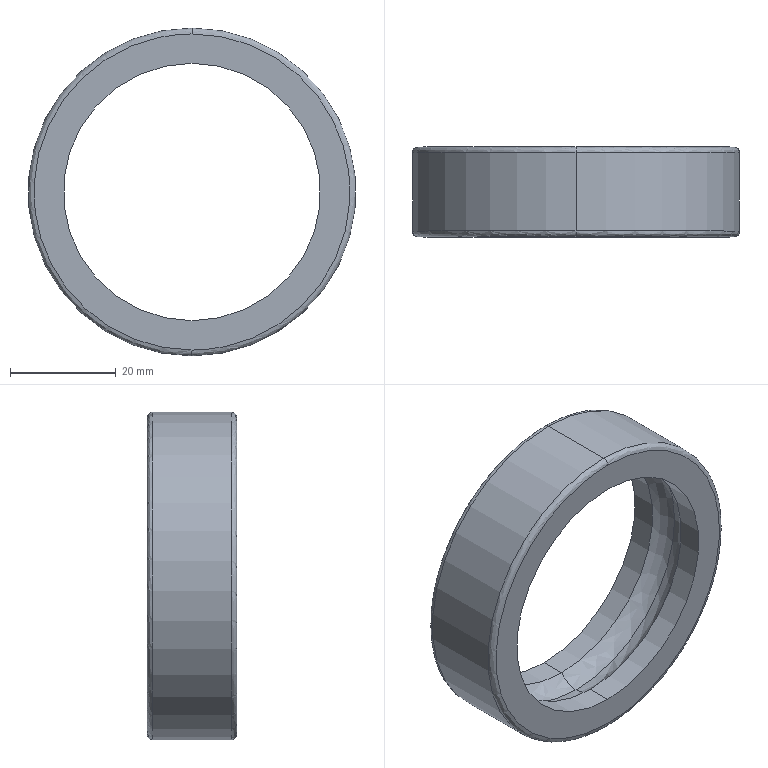Part | SolidWorks | features BaseBody 1 | 1 solid | 16 faces | box 62 x 17 x 62 mm | volume 17853 mm3 | spline 8 | cylinder 6 | plane 2 | commonest cylinder face diameters 48.68 x4 62 x2
STEP:
#1=CARTESIAN_POINT('',(0.,-8.5,29.9));
#2=VERTEX_POINT('',#1);
#3=CARTESIAN_POINT('',(0.,-8.5,-29.9));
#4=VERTEX_POINT('',#3);
#5=CARTESIAN_POINT('',(0.,-8.5,29.9));
#6=CARTESIAN_POINT('',(59.8,-8.5,29.9));
#7=CARTESIAN_POINT('',(59.8,-8.5,-29.9));
#8=CARTESIAN_POINT('',(0.,-8.5,-29.9));
#9=(BOUNDED_CURVE()B_SPLINE_CURVE(3,(#5,#6,#7,#8),.UNSPECIFIED.,.F.,.F.)B_SPLINE_CURVE_WITH_KNOTS((4,4),(0.,1.),.UNSPECIFIED.)CURVE()GEOMETRIC_REPRESENTATION_ITEM()RATIONAL_B_SPLINE_CURVE((1.,0.3333,0.3333,1.))REPRESENTATION_ITEM(''));
#10=EDGE_CURVE('',#2,#4,#9,.T.);
#11=ORIENTED_EDGE('',*,*,#10,.T.);
#12=CARTESIAN_POINT('',(0.,-7.4,-31.));
#13=VERTEX_POINT('',#12);
#14=CARTESIAN_POINT('',(0.,-7.4,-29.9));
#15=DIRECTION('',(1.,0.,0.));
#16=DIRECTION('',(0.,0.,-1.));
#17=AXIS2_PLACEMENT_3D('',#14,#15,#16);
#18=CIRCLE('',#17,1.1);
#19=EDGE_CURVE('',#4,#13,#18,.T.);
#20=ORIENTED_EDGE('',*,*,#19,.T.);
#21=CARTESIAN_POINT('',(0.,-7.4,31.));
#22=VERTEX_POINT('',#21);
#23=CARTESIAN_POINT('',(0.,-7.4,0.));
#24=DIRECTION('',(0.,1.,0.));
#25=DIRECTION('',(0.,0.,-1.));
#26=AXIS2_PLACEMENT_3D('',#23,#24,#25);
#27=CIRCLE('',#26,31.);
#28=EDGE_CURVE('',#22,#13,#27,.T.);
#29=ORIENTED_EDGE('',*,*,#28,.F.);
#30=CARTESIAN_POINT('',(0.,-7.4,29.9));
#31=DIRECTION('',(-1.,0.,0.));
#32=DIRECTION('',(0.,0.,1.));
#33=AXIS2_PLACEMENT_3D('',#30,#31,#32);
#34=CIRCLE('',#33,1.1);
#35=EDGE_CURVE('',#2,#22,#34,.T.);
#36=ORIENTED_EDGE('',*,*,#35,.F.);
#37=EDGE_LOOP('',(#11,#20,#29,#36));
#38=FACE_OUTER_BOUND('',#37,.T.);
#39=CARTESIAN_POINT('',(0.,-8.5,-29.9));
#40=CARTESIAN_POINT('',(59.8,-8.5,-29.9));
#41=CARTESIAN_POINT('',(59.8,-8.5,29.9));
#42=CARTESIAN_POINT('',(0.,-8.5,29.9));
#43=CARTESIAN_POINT('',(0.,-8.5,-30.544));
#44=CARTESIAN_POINT('',(61.089,-8.5,-30.544));
#45=CARTESIAN_POINT('',(61.089,-8.5,30.544));
#46=CARTESIAN_POINT('',(0.,-8.5,30.544));
#47=CARTESIAN_POINT('',(0.,-8.044,-31.));
#48=CARTESIAN_POINT('',(62.,-8.044,-31.));
#49=CARTESIAN_POINT('',(62.,-8.044,31.));
#50=CARTESIAN_POINT('',(0.,-8.044,31.));
#51=CARTESIAN_POINT('',(0.,-7.4,-31.));
#52=CARTESIAN_POINT('',(62.,-7.4,-31.));
#53=CARTESIAN_POINT('',(62.,-7.4,31.));
#54=CARTESIAN_POINT('',(0.,-7.4,31.));
#55=(BOUNDED_SURFACE()B_SPLINE_SURFACE(3,3,((#39,#40,#41,#42),(#43,#44,#45,#46),(#47,#48,#49,#50),(#51,#52,#53,#54)),.UNSPECIFIED.,.F.,.F.,.T.)B_SPLINE_SURFACE_WITH_KNOTS((4,4),(4,4),(0.,1.),(0.,1.),.UNSPECIFIED.)GEOMETRIC_REPRESENTATION_ITEM()RATIONAL_B_SPLINE_SURFACE(((1.,0.3333,0.3333,1.),(0.8047,0.2682,0.2682,0.8047),(0.8047,0.2682,0.2682,0.8047),(1.,0.3333,0.3333,1.)))REPRESENTATION_ITEM('')SURFACE());
#56=ADVANCED_FACE('',(#38),#55,.T.);
#57=CARTESIAN_POINT('',(0.,7.4,-31.));
#58=VERTEX_POINT('',#57);
#59=CARTESIAN_POINT('',(0.,7.4,31.));
#60=VERTEX_POINT('',#59);
#61=CARTESIAN_POINT('',(0.,7.4,0.));
#62=DIRECTION('',(0.,-1.,0.));
#63=DIRECTION('',(0.,0.,-1.));
#64=AXIS2_PLACEMENT_3D('',#61,#62,#63);
#65=CIRCLE('',#64,31.);
#66=EDGE_CURVE('',#58,#60,#65,.T.);
#67=ORIENTED_EDGE('',*,*,#66,.F.);
#68=CARTESIAN_POINT('',(0.,8.5,-29.9));
#69=VERTEX_POINT('',#68);
#70=CARTESIAN_POINT('',(0.,7.4,-29.9));
#71=DIRECTION('',(1.,0.,0.));
#72=DIRECTION('',(0.,0.,-1.));
#73=AXIS2_PLACEMENT_3D('',#70,#71,#72);
#74=CIRCLE('',#73,1.1);
#75=EDGE_CURVE('',#58,#69,#74,.T.);
#76=ORIENTED_EDGE('',*,*,#75,.T.);
#77=CARTESIAN_POINT('',(0.,8.5,29.9));
#78=VERTEX_POINT('',#77);
#79=CARTESIAN_POINT('',(0.,8.5,-29.9));
#80=CARTESIAN_POINT('',(59.8,8.5,-29.9));
#81=CARTESIAN_POINT('',(59.8,8.5,29.9));
#82=CARTESIAN_POINT('',(0.,8.5,29.9));
#83=(BOUNDED_CURVE()B_SPLINE_CURVE(3,(#79,#80,#81,#82),.UNSPECIFIED.,.F.,.F.)B_SPLINE_CURVE_WITH_KNOTS((4,4),(0.,1.),.UNSPECIFIED.)CURVE()GEOMETRIC_REPRESENTATION_ITEM()RATIONAL_B_SPLINE_CURVE((1.,0.3333,0.3333,1.))REPRESENTATION_ITEM(''));
#84=EDGE_CURVE('',#69,#78,#83,.T.);
#85=ORIENTED_EDGE('',*,*,#84,.T.);
#86=CARTESIAN_POINT('',(0.,7.4,29.9));
#87=DIRECTION('',(-1.,0.,0.));
#88=DIRECTION('',(0.,0.,1.));
#89=AXIS2_PLACEMENT_3D('',#86,#87,#88);
#90=CIRCLE('',#89,1.1);
#91=EDGE_CURVE('',#60,#78,#90,.T.);
#92=ORIENTED_EDGE('',*,*,#91,.F.);
#93=EDGE_LOOP('',(#67,#76,#85,#92));
#94=FACE_OUTER_BOUND('',#93,.T.);
#95=CARTESIAN_POINT('',(0.,7.4,-31.));
#96=CARTESIAN_POINT('',(62.,7.4,-31.));
#97=CARTESIAN_POINT('',(62.,7.4,31.));
#98=CARTESIAN_POINT('',(0.,7.4,31.));
#99=CARTESIAN_POINT('',(0.,8.044,-31.));
#100=CARTESIAN_POINT('',(62.,8.044,-31.));
#101=CARTESIAN_POINT('',(62.,8.044,31.));
#102=CARTESIAN_POINT('',(0.,8.044,31.));
#103=CARTESIAN_POINT('',(0.,8.5,-30.544));
#104=CARTESIAN_POINT('',(61.089,8.5,-30.544));
#105=CARTESIAN_POINT('',(61.089,8.5,30.544));
#106=CARTESIAN_POINT('',(0.,8.5,30.544));
#107=CARTESIAN_POINT('',(0.,8.5,-29.9));
#108=CARTESIAN_POINT('',(59.8,8.5,-29.9));
#109=CARTESIAN_POINT('',(59.8,8.5,29.9));
#110=CARTESIAN_POINT('',(0.,8.5,29.9));
#111=(BOUNDED_SURFACE()B_SPLINE_SURFACE(3,3,((#95,#96,#97,#98),(#99,#100,#101,#102),(#103,#104,#105,#106),(#107,#108,#109,#110)),.UNSPECIFIED.,.F.,.F.,.T.)B_SPLINE_SURFACE_WITH_KNOTS((4,4),(4,4),(0.,1.),(0.,1.),.UNSPECIFIED.)GEOMETRIC_REPRESENTATION_ITEM()RATIONAL_B_SPLINE_SURFACE(((1.,0.3333,0.3333,1.),(0.8047,0.2682,0.2682,0.8047),(0.8047,0.2682,0.2682,0.8047),(1.,0.3333,0.3333,1.)))REPRESENTATION_ITEM('')SURFACE());
#112=ADVANCED_FACE('',(#94),#111,.T.);
#113=CARTESIAN_POINT('',(0.,-3.832,24.34));
#114=VERTEX_POINT('',#113);
#115=CARTESIAN_POINT('',(0.,-3.832,-24.34));
#116=VERTEX_POINT('',#115);
#117=CARTESIAN_POINT('',(0.,-3.832,0.));
#118=DIRECTION('',(0.,-1.,0.));
#119=DIRECTION('',(0.,0.,-1.));
#120=AXIS2_PLACEMENT_3D('',#117,#118,#119);
#121=CIRCLE('',#120,24.34);
#122=EDGE_CURVE('',#114,#116,#121,.T.);
#123=ORIENTED_EDGE('',*,*,#122,.T.);
#124=CARTESIAN_POINT('',(0.,0.,-26.375));
#125=VERTEX_POINT('',#124);
#126=CARTESIAN_POINT('',(0.,0.,-21.75));
#127=DIRECTION('',(1.,0.,0.));
#128=DIRECTION('',(0.,0.,-1.));
#129=AXIS2_PLACEMENT_3D('',#126,#127,#128);
#130=CIRCLE('',#129,4.625);
#131=EDGE_CURVE('',#116,#125,#130,.T.);
#132=ORIENTED_EDGE('',*,*,#131,.T.);
#133=CARTESIAN_POINT('',(0.,0.,26.375));
#134=VERTEX_POINT('',#133);
#135=CARTESIAN_POINT('',(0.,0.,0.));
#136=DIRECTION('',(0.,-1.,0.));
#137=DIRECTION('',(0.,0.,1.));
#138=AXIS2_PLACEMENT_3D('',#135,#136,#137);
#139=CIRCLE('',#138,26.375);
#140=EDGE_CURVE('',#134,#125,#139,.T.);
#141=ORIENTED_EDGE('',*,*,#140,.F.);
#142=CARTESIAN_POINT('',(0.,0.,21.75));
#143=DIRECTION('',(-1.,0.,0.));
#144=DIRECTION('',(0.,0.,1.));
#145=AXIS2_PLACEMENT_3D('',#142,#143,#144);
#146=CIRCLE('',#145,4.625);
#147=EDGE_CURVE('',#114,#134,#146,.T.);
#148=ORIENTED_EDGE('',*,*,#147,.F.);
#149=EDGE_LOOP('',(#123,#132,#141,#148));
#150=FACE_OUTER_BOUND('',#149,.T.);
#151=CARTESIAN_POINT('',(0.,-3.832,24.34));
#152=CARTESIAN_POINT('',(-48.68,-3.832,24.34));
#153=CARTESIAN_POINT('',(-48.68,-3.832,-24.34));
#154=CARTESIAN_POINT('',(0.,-3.832,-24.34));
#155=CARTESIAN_POINT('',(0.,-2.953,25.639));
#156=CARTESIAN_POINT('',(-51.279,-2.953,25.639));
#157=CARTESIAN_POINT('',(-51.279,-2.953,-25.639));
#158=CARTESIAN_POINT('',(0.,-2.953,-25.639));
#159=CARTESIAN_POINT('',(0.,-1.568,26.375));
#160=CARTESIAN_POINT('',(-52.75,-1.568,26.375));
#161=CARTESIAN_POINT('',(-52.75,-1.568,-26.375));
#162=CARTESIAN_POINT('',(0.,-1.568,-26.375));
#163=CARTESIAN_POINT('',(0.,0.,26.375));
#164=CARTESIAN_POINT('',(-52.75,0.,26.375));
#165=CARTESIAN_POINT('',(-52.75,0.,-26.375));
#166=CARTESIAN_POINT('',(0.,0.,-26.375));
#167=(BOUNDED_SURFACE()B_SPLINE_SURFACE(3,3,((#151,#152,#153,#154),(#155,#156,#157,#158),(#159,#160,#161,#162),(#163,#164,#165,#166)),.UNSPECIFIED.,.F.,.F.,.F.)B_SPLINE_SURFACE_WITH_KNOTS((4,4),(4,4),(0.,1.),(0.,1.),.UNSPECIFIED.)GEOMETRIC_REPRESENTATION_ITEM()RATIONAL_B_SPLINE_SURFACE(((1.,0.3333,0.3333,1.),(0.9221,0.3074,0.3074,0.9221),(0.9221,0.3074,0.3074,0.9221),(1.,0.3333,0.3333,1.)))REPRESENTATION_ITEM('')SURFACE());
#168=ADVANCED_FACE('',(#150),#167,.F.);
#169=ORIENTED_EDGE('',*,*,#140,.T.);
#170=CARTESIAN_POINT('',(0.,3.832,-24.34));
#171=VERTEX_POINT('',#170);
#172=CARTESIAN_POINT('',(0.,0.,-21.75));
#173=DIRECTION('',(1.,0.,0.));
#174=DIRECTION('',(0.,0.,-1.));
#175=AXIS2_PLACEMENT_3D('',#172,#173,#174);
#176=CIRCLE('',#175,4.625);
#177=EDGE_CURVE('',#125,#171,#176,.T.);
#178=ORIENTED_EDGE('',*,*,#177,.T.);
#179=CARTESIAN_POINT('',(0.,3.832,24.34));
#180=VERTEX_POINT('',#179);
#181=CARTESIAN_POINT('',(0.,3.832,0.));
#182=DIRECTION('',(0.,1.,0.));
#183=DIRECTION('',(0.,0.,-1.));
#184=AXIS2_PLACEMENT_3D('',#181,#182,#183);
#185=CIRCLE('',#184,24.34);
#186=EDGE_CURVE('',#171,#180,#185,.T.);
#187=ORIENTED_EDGE('',*,*,#186,.T.);
#188=CARTESIAN_POINT('',(0.,0.,21.75));
#189=DIRECTION('',(-1.,0.,0.));
#190=DIRECTION('',(0.,0.,1.));
#191=AXIS2_PLACEMENT_3D('',#188,#189,#190);
#192=CIRCLE('',#191,4.625);
#193=EDGE_CURVE('',#134,#180,#192,.T.);
#194=ORIENTED_EDGE('',*,*,#193,.F.);
#195=EDGE_LOOP('',(#169,#178,#187,#194));
#196=FACE_OUTER_BOUND('',#195,.T.);
#197=CARTESIAN_POINT('',(0.,0.,26.375));
#198=CARTESIAN_POINT('',(-52.75,0.,26.375));
#199=CARTESIAN_POINT('',(-52.75,0.,-26.375));
#200=CARTESIAN_POINT('',(0.,0.,-26.375));
#201=CARTESIAN_POINT('',(0.,1.568,26.375));
#202=CARTESIAN_POINT('',(-52.75,1.568,26.375));
#203=CARTESIAN_POINT('',(-52.75,1.568,-26.375));
#204=CARTESIAN_POINT('',(0.,1.568,-26.375));
#205=CARTESIAN_POINT('',(0.,2.953,25.639));
#206=CARTESIAN_POINT('',(-51.279,2.953,25.639));
#207=CARTESIAN_POINT('',(-51.279,2.953,-25.639));
#208=CARTESIAN_POINT('',(0.,2.953,-25.639));
#209=CARTESIAN_POINT('',(0.,3.832,24.34));
#210=CARTESIAN_POINT('',(-48.68,3.832,24.34));
#211=CARTESIAN_POINT('',(-48.68,3.832,-24.34));
#212=CARTESIAN_POINT('',(0.,3.832,-24.34));
#213=(BOUNDED_SURFACE()B_SPLINE_SURFACE(3,3,((#197,#198,#199,#200),(#201,#202,#203,#204),(#205,#206,#207,#208),(#209,#210,#211,#212)),.UNSPECIFIED.,.F.,.F.,.T.)B_SPLINE_SURFACE_WITH_KNOTS((4,4),(4,4),(0.,1.),(0.,1.),.UNSPECIFIED.)GEOMETRIC_REPRESENTATION_ITEM()RATIONAL_B_SPLINE_SURFACE(((1.,0.3333,0.3333,1.),(0.9221,0.3074,0.3074,0.9221),(0.9221,0.3074,0.3074,0.9221),(1.,0.3333,0.3333,1.)))REPRESENTATION_ITEM('')SURFACE());
#214=ADVANCED_FACE('',(#196),#213,.F.);
#215=ORIENTED_EDGE('',*,*,#66,.T.);
#216=CARTESIAN_POINT('',(0.,9.35,31.));
#217=DIRECTION('',(0.,-1.,0.));
#218=VECTOR('',#217,1000.);
#219=LINE('',#216,#218);
#220=EDGE_CURVE('',#60,#22,#219,.T.);
#221=ORIENTED_EDGE('',*,*,#220,.T.);
#222=ORIENTED_EDGE('',*,*,#28,.T.);
#223=CARTESIAN_POINT('',(0.,9.35,-31.));
#224=DIRECTION('',(0.,-1.,0.));
#225=VECTOR('',#224,1000.);
#226=LINE('',#223,#225);
#227=EDGE_CURVE('',#58,#13,#226,.T.);
#228=ORIENTED_EDGE('',*,*,#227,.F.);
#229=EDGE_LOOP('',(#215,#221,#222,#228));
#230=FACE_OUTER_BOUND('',#229,.T.);
#231=CARTESIAN_POINT('',(0.,9.35,0.));
#232=DIRECTION('',(0.,-1.,0.));
#233=DIRECTION('',(0.,0.,-1.));
#234=AXIS2_PLACEMENT_3D('',#231,#232,#233);
#235=CYLINDRICAL_SURFACE('',#234,31.);
#236=ADVANCED_FACE('',(#230),#235,.T.);
#237=ORIENTED_EDGE('',*,*,#122,.F.);
#238=CARTESIAN_POINT('',(0.,-8.5,24.34));
#239=VERTEX_POINT('',#238);
#240=CARTESIAN_POINT('',(0.,9.35,24.34));
#241=DIRECTION('',(0.,-1.,0.));
#242=VECTOR('',#241,1000.);
#243=LINE('',#240,#242);
#244=EDGE_CURVE('',#114,#239,#243,.T.);
#245=ORIENTED_EDGE('',*,*,#244,.T.);
#246=CARTESIAN_POINT('',(0.,-8.5,-24.34));
#247=VERTEX_POINT('',#246);
#248=CARTESIAN_POINT('',(0.,-8.5,0.));
#249=DIRECTION('',(0.,1.,0.));
#250=DIRECTION('',(0.,0.,-1.));
#251=AXIS2_PLACEMENT_3D('',#248,#249,#250);
#252=CIRCLE('',#251,24.34);
#253=EDGE_CURVE('',#247,#239,#252,.T.);
#254=ORIENTED_EDGE('',*,*,#253,.F.);
#255=CARTESIAN_POINT('',(0.,9.35,-24.34));
#256=DIRECTION('',(0.,-1.,0.));
#257=VECTOR('',#256,1000.);
#258=LINE('',#255,#257);
#259=EDGE_CURVE('',#116,#247,#258,.T.);
#260=ORIENTED_EDGE('',*,*,#259,.F.);
#261=EDGE_LOOP('',(#237,#245,#254,#260));
#262=FACE_OUTER_BOUND('',#261,.T.);
#263=CARTESIAN_POINT('',(0.,9.35,0.));
#264=DIRECTION('',(0.,-1.,0.));
#265=DIRECTION('',(0.,0.,-1.));
#266=AXIS2_PLACEMENT_3D('',#263,#264,#265);
#267=CYLINDRICAL_SURFACE('',#266,24.34);
#268=ADVANCED_FACE('',(#262),#267,.F.);
#269=CARTESIAN_POINT('',(0.,8.5,-24.34));
#270=VERTEX_POINT('',#269);
#271=CARTESIAN_POINT('',(0.,8.5,24.34));
#272=VERTEX_POINT('',#271);
#273=CARTESIAN_POINT('',(0.,8.5,0.));
#274=DIRECTION('',(0.,1.,0.));
#275=DIRECTION('',(0.,0.,-1.));
#276=AXIS2_PLACEMENT_3D('',#273,#274,#275);
#277=CIRCLE('',#276,24.34);
#278=EDGE_CURVE('',#270,#272,#277,.T.);
#279=ORIENTED_EDGE('',*,*,#278,.T.);
#280=CARTESIAN_POINT('',(0.,9.35,24.34));
#281=DIRECTION('',(0.,-1.,0.));
#282=VECTOR('',#281,1000.);
#283=LINE('',#280,#282);
#284=EDGE_CURVE('',#272,#180,#283,.T.);
#285=ORIENTED_EDGE('',*,*,#284,.T.);
#286=ORIENTED_EDGE('',*,*,#186,.F.);
#287=CARTESIAN_POINT('',(0.,9.35,-24.34));
#288=DIRECTION('',(0.,-1.,0.));
#289=VECTOR('',#288,1000.);
#290=LINE('',#287,#289);
#291=EDGE_CURVE('',#270,#171,#290,.T.);
#292=ORIENTED_EDGE('',*,*,#291,.F.);
#293=EDGE_LOOP('',(#279,#285,#286,#292));
#294=FACE_OUTER_BOUND('',#293,.T.);
#295=CARTESIAN_POINT('',(0.,9.35,0.));
#296=DIRECTION('',(0.,-1.,0.));
#297=DIRECTION('',(0.,0.,-1.));
#298=AXIS2_PLACEMENT_3D('',#295,#296,#297);
#299=CYLINDRICAL_SURFACE('',#298,24.34);
#300=ADVANCED_FACE('',(#294),#299,.F.);
#301=ORIENTED_EDGE('',*,*,#177,.F.);
#302=CARTESIAN_POINT('',(0.,0.,0.));
#303=DIRECTION('',(0.,-1.,0.));
#304=DIRECTION('',(0.,0.,1.));
#305=AXIS2_PLACEMENT_3D('',#302,#303,#304);
#306=CIRCLE('',#305,26.375);
#307=EDGE_CURVE('',#125,#134,#306,.T.);
#308=ORIENTED_EDGE('',*,*,#307,.T.);
#309=ORIENTED_EDGE('',*,*,#193,.T.);
#310=CARTESIAN_POINT('',(0.,3.832,0.));
#311=DIRECTION('',(0.,1.,0.));
#312=DIRECTION('',(0.,0.,-1.));
#313=AXIS2_PLACEMENT_3D('',#310,#311,#312);
#314=CIRCLE('',#313,24.34);
#315=EDGE_CURVE('',#180,#171,#314,.T.);
#316=ORIENTED_EDGE('',*,*,#315,.T.);
#317=EDGE_LOOP('',(#301,#308,#309,#316));
#318=FACE_OUTER_BOUND('',#317,.T.);
#319=CARTESIAN_POINT('',(0.,0.,-26.375));
#320=CARTESIAN_POINT('',(52.75,0.,-26.375));
#321=CARTESIAN_POINT('',(52.75,0.,26.375));
#322=CARTESIAN_POINT('',(0.,0.,26.375));
#323=CARTESIAN_POINT('',(0.,1.568,-26.375));
#324=CARTESIAN_POINT('',(52.75,1.568,-26.375));
#325=CARTESIAN_POINT('',(52.75,1.568,26.375));
#326=CARTESIAN_POINT('',(0.,1.568,26.375));
#327=CARTESIAN_POINT('',(0.,2.953,-25.639));
#328=CARTESIAN_POINT('',(51.279,2.953,-25.639));
#329=CARTESIAN_POINT('',(51.279,2.953,25.639));
#330=CARTESIAN_POINT('',(0.,2.953,25.639));
#331=CARTESIAN_POINT('',(0.,3.832,-24.34));
#332=CARTESIAN_POINT('',(48.68,3.832,-24.34));
#333=CARTESIAN_POINT('',(48.68,3.832,24.34));
#334=CARTESIAN_POINT('',(0.,3.832,24.34));
#335=(BOUNDED_SURFACE()B_SPLINE_SURFACE(3,3,((#319,#320,#321,#322),(#323,#324,#325,#326),(#327,#328,#329,#330),(#331,#332,#333,#334)),.UNSPECIFIED.,.F.,.F.,.T.)B_SPLINE_SURFACE_WITH_KNOTS((4,4),(4,4),(0.,1.),(0.,1.),.UNSPECIFIED.)GEOMETRIC_REPRESENTATION_ITEM()RATIONAL_B_SPLINE_SURFACE(((1.,0.3333,0.3333,1.),(0.9221,0.3074,0.3074,0.9221),(0.9221,0.3074,0.3074,0.9221),(1.,0.3333,0.3333,1.)))REPRESENTATION_ITEM('')SURFACE());
#336=ADVANCED_FACE('',(#318),#335,.F.);
#337=ORIENTED_EDGE('',*,*,#220,.F.);
#338=CARTESIAN_POINT('',(0.,7.4,0.));
#339=DIRECTION('',(0.,-1.,0.));
#340=DIRECTION('',(0.,0.,-1.));
#341=AXIS2_PLACEMENT_3D('',#338,#339,#340);
#342=CIRCLE('',#341,31.);
#343=EDGE_CURVE('',#60,#58,#342,.T.);
#344=ORIENTED_EDGE('',*,*,#343,.T.);
#345=ORIENTED_EDGE('',*,*,#227,.T.);
#346=CARTESIAN_POINT('',(0.,-7.4,0.));
#347=DIRECTION('',(0.,1.,0.));
#348=DIRECTION('',(0.,0.,-1.));
#349=AXIS2_PLACEMENT_3D('',#346,#347,#348);
#350=CIRCLE('',#349,31.);
#351=EDGE_CURVE('',#13,#22,#350,.T.);
#352=ORIENTED_EDGE('',*,*,#351,.T.);
#353=EDGE_LOOP('',(#337,#344,#345,#352));
#354=FACE_OUTER_BOUND('',#353,.T.);
#355=CARTESIAN_POINT('',(0.,9.35,0.));
#356=DIRECTION('',(0.,-1.,0.));
#357=DIRECTION('',(0.,0.,-1.));
#358=AXIS2_PLACEMENT_3D('',#355,#356,#357);
#359=CYLINDRICAL_SURFACE('',#358,31.);
#360=ADVANCED_FACE('',(#354),#359,.T.);
#361=ORIENTED_EDGE('',*,*,#19,.F.);
#362=CARTESIAN_POINT('',(0.,-8.5,-29.9));
#363=CARTESIAN_POINT('',(-59.8,-8.5,-29.9));
#364=CARTESIAN_POINT('',(-59.8,-8.5,29.9));
#365=CARTESIAN_POINT('',(0.,-8.5,29.9));
#366=(BOUNDED_CURVE()B_SPLINE_CURVE(3,(#362,#363,#364,#365),.UNSPECIFIED.,.F.,.F.)B_SPLINE_CURVE_WITH_KNOTS((4,4),(0.,1.),.UNSPECIFIED.)CURVE()GEOMETRIC_REPRESENTATION_ITEM()RATIONAL_B_SPLINE_CURVE((1.,0.3333,0.3333,1.))REPRESENTATION_ITEM(''));
#367=EDGE_CURVE('',#4,#2,#366,.T.);
#368=ORIENTED_EDGE('',*,*,#367,.T.);
#369=ORIENTED_EDGE('',*,*,#35,.T.);
#370=ORIENTED_EDGE('',*,*,#351,.F.);
#371=EDGE_LOOP('',(#361,#368,#369,#370));
#372=FACE_OUTER_BOUND('',#371,.T.);
#373=CARTESIAN_POINT('',(0.,-8.5,29.9));
#374=CARTESIAN_POINT('',(-59.8,-8.5,29.9));
#375=CARTESIAN_POINT('',(-59.8,-8.5,-29.9));
#376=CARTESIAN_POINT('',(0.,-8.5,-29.9));
#377=CARTESIAN_POINT('',(0.,-8.5,30.544));
#378=CARTESIAN_POINT('',(-61.089,-8.5,30.544));
#379=CARTESIAN_POINT('',(-61.089,-8.5,-30.544));
#380=CARTESIAN_POINT('',(0.,-8.5,-30.544));
#381=CARTESIAN_POINT('',(0.,-8.044,31.));
#382=CARTESIAN_POINT('',(-62.,-8.044,31.));
#383=CARTESIAN_POINT('',(-62.,-8.044,-31.));
#384=CARTESIAN_POINT('',(0.,-8.044,-31.));
#385=CARTESIAN_POINT('',(0.,-7.4,31.));
#386=CARTESIAN_POINT('',(-62.,-7.4,31.));
#387=CARTESIAN_POINT('',(-62.,-7.4,-31.));
#388=CARTESIAN_POINT('',(0.,-7.4,-31.));
#389=(BOUNDED_SURFACE()B_SPLINE_SURFACE(3,3,((#373,#374,#375,#376),(#377,#378,#379,#380),(#381,#382,#383,#384),(#385,#386,#387,#388)),.UNSPECIFIED.,.F.,.F.,.F.)B_SPLINE_SURFACE_WITH_KNOTS((4,4),(4,4),(0.,1.),(0.,1.),.UNSPECIFIED.)GEOMETRIC_REPRESENTATION_ITEM()RATIONAL_B_SPLINE_SURFACE(((1.,0.3333,0.3333,1.),(0.8047,0.2682,0.2682,0.8047),(0.8047,0.2682,0.2682,0.8047),(1.,0.3333,0.3333,1.)))REPRESENTATION_ITEM('')SURFACE());
#390=ADVANCED_FACE('',(#372),#389,.T.);
#391=ORIENTED_EDGE('',*,*,#75,.F.);
#392=ORIENTED_EDGE('',*,*,#343,.F.);
#393=ORIENTED_EDGE('',*,*,#91,.T.);
#394=CARTESIAN_POINT('',(0.,8.5,29.9));
#395=CARTESIAN_POINT('',(-59.8,8.5,29.9));
#396=CARTESIAN_POINT('',(-59.8,8.5,-29.9));
#397=CARTESIAN_POINT('',(0.,8.5,-29.9));
#398=(BOUNDED_CURVE()B_SPLINE_CURVE(3,(#394,#395,#396,#397),.UNSPECIFIED.,.F.,.T.)B_SPLINE_CURVE_WITH_KNOTS((4,4),(0.,1.),.UNSPECIFIED.)CURVE()GEOMETRIC_REPRESENTATION_ITEM()RATIONAL_B_SPLINE_CURVE((1.,0.3333,0.3333,1.))REPRESENTATION_ITEM(''));
#399=EDGE_CURVE('',#78,#69,#398,.T.);
#400=ORIENTED_EDGE('',*,*,#399,.T.);
#401=EDGE_LOOP('',(#391,#392,#393,#400));
#402=FACE_OUTER_BOUND('',#401,.T.);
#403=CARTESIAN_POINT('',(0.,7.4,31.));
#404=CARTESIAN_POINT('',(-62.,7.4,31.));
#405=CARTESIAN_POINT('',(-62.,7.4,-31.));
#406=CARTESIAN_POINT('',(0.,7.4,-31.));
#407=CARTESIAN_POINT('',(0.,8.044,31.));
#408=CARTESIAN_POINT('',(-62.,8.044,31.));
#409=CARTESIAN_POINT('',(-62.,8.044,-31.));
#410=CARTESIAN_POINT('',(0.,8.044,-31.));
#411=CARTESIAN_POINT('',(0.,8.5,30.544));
#412=CARTESIAN_POINT('',(-61.089,8.5,30.544));
#413=CARTESIAN_POINT('',(-61.089,8.5,-30.544));
#414=CARTESIAN_POINT('',(0.,8.5,-30.544));
#415=CARTESIAN_POINT('',(0.,8.5,29.9));
#416=CARTESIAN_POINT('',(-59.8,8.5,29.9));
#417=CARTESIAN_POINT('',(-59.8,8.5,-29.9));
#418=CARTESIAN_POINT('',(0.,8.5,-29.9));
#419=(BOUNDED_SURFACE()B_SPLINE_SURFACE(3,3,((#403,#404,#405,#406),(#407,#408,#409,#410),(#411,#412,#413,#414),(#415,#416,#417,#418)),.UNSPECIFIED.,.F.,.F.,.T.)B_SPLINE_SURFACE_WITH_KNOTS((4,4),(4,4),(0.,1.),(0.,1.),.UNSPECIFIED.)GEOMETRIC_REPRESENTATION_ITEM()RATIONAL_B_SPLINE_SURFACE(((1.,0.3333,0.3333,1.),(0.8047,0.2682,0.2682,0.8047),(0.8047,0.2682,0.2682,0.8047),(1.,0.3333,0.3333,1.)))REPRESENTATION_ITEM('')SURFACE());
#420=ADVANCED_FACE('',(#402),#419,.T.);
#421=ORIENTED_EDGE('',*,*,#253,.T.);
#422=CARTESIAN_POINT('',(0.,-8.5,0.));
#423=DIRECTION('',(0.,1.,0.));
#424=DIRECTION('',(0.,0.,-1.));
#425=AXIS2_PLACEMENT_3D('',#422,#423,#424);
#426=CIRCLE('',#425,24.34);
#427=EDGE_CURVE('',#239,#247,#426,.T.);
#428=ORIENTED_EDGE('',*,*,#427,.T.);
#429=EDGE_LOOP('',(#421,#428));
#430=FACE_BOUND('',#429,.T.);
#431=ORIENTED_EDGE('',*,*,#367,.F.);
#432=ORIENTED_EDGE('',*,*,#10,.F.);
#433=EDGE_LOOP('',(#431,#432));
#434=FACE_OUTER_BOUND('',#433,.T.);
#435=CARTESIAN_POINT('',(0.,-8.5,0.));
#436=DIRECTION('',(0.,-1.,0.));
#437=DIRECTION('',(0.,0.,-1.));
#438=AXIS2_PLACEMENT_3D('',#435,#436,#437);
#439=PLANE('',#438);
#440=ADVANCED_FACE('',(#430,#434),#439,.T.);
#441=ORIENTED_EDGE('',*,*,#278,.F.);
#442=CARTESIAN_POINT('',(0.,8.5,0.));
#443=DIRECTION('',(0.,1.,0.));
#444=DIRECTION('',(0.,0.,-1.));
#445=AXIS2_PLACEMENT_3D('',#442,#443,#444);
#446=CIRCLE('',#445,24.34);
#447=EDGE_CURVE('',#272,#270,#446,.T.);
#448=ORIENTED_EDGE('',*,*,#447,.F.);
#449=EDGE_LOOP('',(#441,#448));
#450=FACE_BOUND('',#449,.T.);
#451=ORIENTED_EDGE('',*,*,#399,.F.);
#452=ORIENTED_EDGE('',*,*,#84,.F.);
#453=EDGE_LOOP('',(#451,#452));
#454=FACE_OUTER_BOUND('',#453,.T.);
#455=CARTESIAN_POINT('',(0.,8.5,0.));
#456=DIRECTION('',(0.,-1.,0.));
#457=DIRECTION('',(0.,0.,-1.));
#458=AXIS2_PLACEMENT_3D('',#455,#456,#457);
#459=PLANE('',#458);
#460=ADVANCED_FACE('',(#450,#454),#459,.F.);
#461=ORIENTED_EDGE('',*,*,#244,.F.);
#462=CARTESIAN_POINT('',(0.,-3.832,0.));
#463=DIRECTION('',(0.,-1.,0.));
#464=DIRECTION('',(0.,0.,-1.));
#465=AXIS2_PLACEMENT_3D('',#462,#463,#464);
#466=CIRCLE('',#465,24.34);
#467=EDGE_CURVE('',#116,#114,#466,.T.);
#468=ORIENTED_EDGE('',*,*,#467,.F.);
#469=ORIENTED_EDGE('',*,*,#259,.T.);
#470=ORIENTED_EDGE('',*,*,#427,.F.);
#471=EDGE_LOOP('',(#461,#468,#469,#470));
#472=FACE_OUTER_BOUND('',#471,.T.);
#473=CARTESIAN_POINT('',(0.,9.35,0.));
#474=DIRECTION('',(0.,-1.,0.));
#475=DIRECTION('',(0.,0.,-1.));
#476=AXIS2_PLACEMENT_3D('',#473,#474,#475);
#477=CYLINDRICAL_SURFACE('',#476,24.34);
#478=ADVANCED_FACE('',(#472),#477,.F.);
#479=ORIENTED_EDGE('',*,*,#284,.F.);
#480=ORIENTED_EDGE('',*,*,#447,.T.);
#481=ORIENTED_EDGE('',*,*,#291,.T.);
#482=ORIENTED_EDGE('',*,*,#315,.F.);
#483=EDGE_LOOP('',(#479,#480,#481,#482));
#484=FACE_OUTER_BOUND('',#483,.T.);
#485=CARTESIAN_POINT('',(0.,9.35,0.));
#486=DIRECTION('',(0.,-1.,0.));
#487=DIRECTION('',(0.,0.,-1.));
#488=AXIS2_PLACEMENT_3D('',#485,#486,#487);
#489=CYLINDRICAL_SURFACE('',#488,24.34);
#490=ADVANCED_FACE('',(#484),#489,.F.);
#491=ORIENTED_EDGE('',*,*,#131,.F.);
#492=ORIENTED_EDGE('',*,*,#467,.T.);
#493=ORIENTED_EDGE('',*,*,#147,.T.);
#494=ORIENTED_EDGE('',*,*,#307,.F.);
#495=EDGE_LOOP('',(#491,#492,#493,#494));
#496=FACE_OUTER_BOUND('',#495,.T.);
#497=CARTESIAN_POINT('',(0.,-3.832,-24.34));
#498=CARTESIAN_POINT('',(48.68,-3.832,-24.34));
#499=CARTESIAN_POINT('',(48.68,-3.832,24.34));
#500=CARTESIAN_POINT('',(0.,-3.832,24.34));
#501=CARTESIAN_POINT('',(0.,-2.953,-25.639));
#502=CARTESIAN_POINT('',(51.279,-2.953,-25.639));
#503=CARTESIAN_POINT('',(51.279,-2.953,25.639));
#504=CARTESIAN_POINT('',(0.,-2.953,25.639));
#505=CARTESIAN_POINT('',(0.,-1.568,-26.375));
#506=CARTESIAN_POINT('',(52.75,-1.568,-26.375));
#507=CARTESIAN_POINT('',(52.75,-1.568,26.375));
#508=CARTESIAN_POINT('',(0.,-1.568,26.375));
#509=CARTESIAN_POINT('',(0.,0.,-26.375));
#510=CARTESIAN_POINT('',(52.75,0.,-26.375));
#511=CARTESIAN_POINT('',(52.75,0.,26.375));
#512=CARTESIAN_POINT('',(0.,0.,26.375));
#513=(BOUNDED_SURFACE()B_SPLINE_SURFACE(3,3,((#497,#498,#499,#500),(#501,#502,#503,#504),(#505,#506,#507,#508),(#509,#510,#511,#512)),.UNSPECIFIED.,.F.,.F.,.T.)B_SPLINE_SURFACE_WITH_KNOTS((4,4),(4,4),(0.,1.),(0.,1.),.UNSPECIFIED.)GEOMETRIC_REPRESENTATION_ITEM()RATIONAL_B_SPLINE_SURFACE(((1.,0.3333,0.3333,1.),(0.9221,0.3074,0.3074,0.9221),(0.9221,0.3074,0.3074,0.9221),(1.,0.3333,0.3333,1.)))REPRESENTATION_ITEM('')SURFACE());
#514=ADVANCED_FACE('',(#496),#513,.F.);
#515=CLOSED_SHELL('',(#56,#112,#168,#214,#236,#268,#300,#336,#360,#390,#420,#440,#460,#478,#490,#514));
#516=MANIFOLD_SOLID_BREP('',#515);
#517=CARTESIAN_POINT('',(0.,0.,0.));
#518=DIRECTION('',(0.,0.,1.));
#519=DIRECTION('',(1.,0.,0.));
#520=AXIS2_PLACEMENT_3D('',#517,#518,#519);
#521=(LENGTH_UNIT()NAMED_UNIT(*)SI_UNIT(.MILLI.,.METRE.));
#522=UNCERTAINTY_MEASURE_WITH_UNIT(LENGTH_MEASURE(0.00001),#521,'','');
#523=(NAMED_UNIT(*)PLANE_ANGLE_UNIT()SI_UNIT($,.RADIAN.));
#524=(NAMED_UNIT(*)SI_UNIT($,.STERADIAN.)SOLID_ANGLE_UNIT());
#525=(GEOMETRIC_REPRESENTATION_CONTEXT(3)GLOBAL_UNCERTAINTY_ASSIGNED_CONTEXT((#522))GLOBAL_UNIT_ASSIGNED_CONTEXT((#521,#523,#524))REPRESENTATION_CONTEXT('',''));
#526=ADVANCED_BREP_SHAPE_REPRESENTATION('',(#516,#520),#525);